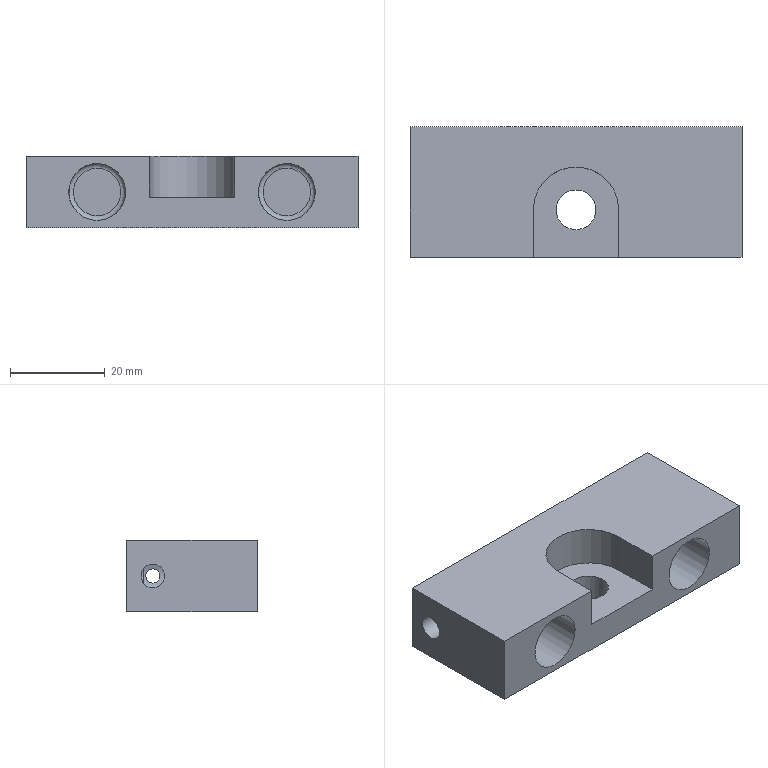NC program | NX | posted with a generic post | part box 70 x 27.5 x 15 mm
Lines 1624 to 2444 of 3352:
(PLANAR_MILL_2 , TOOL : D4-12-D4-50-3T-ROUGH)
N3228 T03 M6
N3230 G53
N3232 G17 G0 G90 X-5.038 Y-1.722 B0. C0. S3000 M3
N3234 G43 Z20. H3
N3236 Z-7.6
N3238 G94 G1 X-5.003 Y-1.751 Z-7.601 F600.
N3240 X-4.742 Y-1.911 Z-7.606
N3242 X-4.462 Y-2.032 Z-7.611
N3244 X-4.167 Y-2.112 Z-7.617
N3246 X-3.864 Y-2.15 Z-7.622
N3248 X-3.636 Z-7.626
N3250 X-3.333 Y-2.112 Z-7.631
N3252 X-3.038 Y-2.032 Z-7.637
N3254 X-2.758 Y-1.911 Z-7.642
N3256 X-2.497 Y-1.751 Z-7.647
N3258 X-2.262 Y-1.556 Z-7.653
N3260 X-2.057 Y-1.33 Z-7.658
N3262 X-1.885 Y-1.077 Z-7.663
N3264 X-1.752 Y-0.802 Z-7.669
N3266 X-1.658 Y-0.511 Z-7.674
N3268 X-1.607 Y-0.209 Z-7.679
N3270 X-1.599 Y0.096 Z-7.685
N3272 X-1.634 Y0.4 Z-7.69
N3274 X-1.712 Y0.695 Z-7.695
N3276 X-1.831 Y0.977 Z-7.701
N3278 X-1.945 Y1.173 Z-7.705
N3280 X-2.119 Y1.405 Z-7.71
N3282 X-2.322 Y1.611 Z-7.715
N3284 X-2.551 Y1.788 Z-7.72
N3286 X-2.801 Y1.933 Z-7.725
N3288 X-3.069 Y2.042 Z-7.73
N3290 X-3.349 Y2.115 Z-7.735
N3292 X-3.636 Y2.15 Z-7.74
N3294 X-3.864 Z-7.744
N3296 X-4.151 Y2.115 Z-7.749
N3298 X-4.431 Y2.042 Z-7.754
N3300 X-4.699 Y1.933 Z-7.759
N3302 X-4.949 Y1.788 Z-7.764
N3304 X-5.178 Y1.611 Z-7.769
N3306 X-5.381 Y1.405 Z-7.774
N3308 X-5.555 Y1.173 Z-7.779
N3310 X-5.669 Y0.977 Z-7.783
N3312 X-5.788 Y0.695 Z-7.789
N3314 X-5.866 Y0.4 Z-7.794
N3316 X-5.901 Y0.096 Z-7.799
N3318 X-5.893 Y-0.209 Z-7.805
N3320 X-5.842 Y-0.511 Z-7.81
N3322 X-5.748 Y-0.802 Z-7.815
N3324 X-5.615 Y-1.077 Z-7.821
N3326 X-5.443 Y-1.33 Z-7.826
N3328 X-5.238 Y-1.556 Z-7.831
N3330 X-5.003 Y-1.751 Z-7.837
N3332 X-4.742 Y-1.911 Z-7.842
N3334 X-4.462 Y-2.032 Z-7.847
N3336 X-4.167 Y-2.112 Z-7.853
N3338 X-3.864 Y-2.15 Z-7.858
N3340 X-3.636 Z-7.862
N3342 X-3.333 Y-2.112 Z-7.867
N3344 X-3.038 Y-2.032 Z-7.873
N3346 X-2.758 Y-1.911 Z-7.878
N3348 X-2.497 Y-1.751 Z-7.883
N3350 X-2.262 Y-1.556 Z-7.889
N3352 X-2.057 Y-1.33 Z-7.894
N3354 X-1.885 Y-1.077 Z-7.899
N3356 X-1.752 Y-0.802 Z-7.905
N3358 X-1.658 Y-0.511 Z-7.91
N3360 X-1.607 Y-0.209 Z-7.915
N3362 X-1.599 Y0.096 Z-7.921
N3364 X-1.634 Y0.4 Z-7.926
N3366 X-1.712 Y0.695 Z-7.931
N3368 X-1.831 Y0.977 Z-7.937
N3370 X-1.945 Y1.173 Z-7.941
N3372 X-2.119 Y1.405 Z-7.946
N3374 X-2.322 Y1.611 Z-7.951
N3376 X-2.551 Y1.788 Z-7.956
N3378 X-2.801 Y1.933 Z-7.961
N3380 X-3.069 Y2.042 Z-7.966
N3382 X-3.349 Y2.115 Z-7.971
N3384 X-3.636 Y2.15 Z-7.976
N3386 X-3.864 Z-7.98
N3388 X-4.151 Y2.115 Z-7.985
N3390 X-4.431 Y2.042 Z-7.99
N3392 X-4.699 Y1.933 Z-7.995
N3394 X-4.949 Y1.788 Z-8.
N3396 X-5.178 Y1.611 Z-8.005
N3398 X-5.381 Y1.405 Z-8.01
N3400 X-5.555 Y1.173 Z-8.015
N3402 X-5.669 Y0.977 Z-8.019
N3404 X-5.788 Y0.695 Z-8.025
N3406 X-5.866 Y0.4 Z-8.03
N3408 X-5.901 Y0.096 Z-8.035
N3410 X-5.893 Y-0.209 Z-8.041
N3412 X-5.842 Y-0.511 Z-8.046
N3414 X-5.748 Y-0.802 Z-8.051
N3416 X-5.615 Y-1.077 Z-8.057
N3418 X-5.443 Y-1.33 Z-8.062
N3420 X-5.238 Y-1.556 Z-8.067
N3422 X-5.003 Y-1.751 Z-8.073
N3424 X-4.742 Y-1.911 Z-8.078
N3426 X-4.462 Y-2.032 Z-8.083
N3428 X-4.167 Y-2.112 Z-8.089
N3430 X-3.864 Y-2.15 Z-8.094
N3432 X-3.636 Z-8.098
N3434 X-3.333 Y-2.112 Z-8.103
N3436 X-3.038 Y-2.032 Z-8.109
N3438 X-2.758 Y-1.911 Z-8.114
N3440 X-2.497 Y-1.751 Z-8.119
N3442 X-2.262 Y-1.556 Z-8.125
N3444 X-2.057 Y-1.33 Z-8.13
N3446 X-1.885 Y-1.077 Z-8.135
N3448 X-1.752 Y-0.802 Z-8.141
N3450 X-1.658 Y-0.511 Z-8.146
N3452 X-1.607 Y-0.209 Z-8.151
N3454 X-1.599 Y0.096 Z-8.157
N3456 X-1.634 Y0.4 Z-8.162
N3458 X-1.712 Y0.695 Z-8.167
N3460 X-1.831 Y0.977 Z-8.173
N3462 X-1.945 Y1.173 Z-8.177
N3464 X-2.119 Y1.405 Z-8.182
N3466 X-2.322 Y1.611 Z-8.187
N3468 X-2.551 Y1.788 Z-8.192
N3470 X-2.801 Y1.933 Z-8.197
N3472 X-3.069 Y2.042 Z-8.202
N3474 X-3.349 Y2.115 Z-8.207
N3476 X-3.636 Y2.15 Z-8.212
N3478 X-3.864 Z-8.216
N3480 X-4.151 Y2.115 Z-8.221
N3482 X-4.431 Y2.042 Z-8.226
N3484 X-4.699 Y1.933 Z-8.231
N3486 X-4.949 Y1.788 Z-8.236
N3488 X-5.178 Y1.611 Z-8.241
N3490 X-5.381 Y1.405 Z-8.246
N3492 X-5.555 Y1.173 Z-8.251
N3494 X-5.669 Y0.977 Z-8.255
N3496 X-5.788 Y0.695 Z-8.261
N3498 X-5.866 Y0.4 Z-8.266
N3500 X-5.901 Y0.096 Z-8.271
N3502 X-5.893 Y-0.209 Z-8.277
N3504 X-5.842 Y-0.511 Z-8.282
N3506 X-5.748 Y-0.802 Z-8.287
N3508 X-5.615 Y-1.077 Z-8.293
N3510 X-5.443 Y-1.33 Z-8.298
N3512 X-5.238 Y-1.556 Z-8.303
N3514 X-5.003 Y-1.751 Z-8.309
N3516 X-4.742 Y-1.911 Z-8.314
N3518 X-4.462 Y-2.032 Z-8.319
N3520 X-4.167 Y-2.112 Z-8.325
N3522 X-3.864 Y-2.15 Z-8.33
N3524 X-3.636 Z-8.334
N3526 X-3.333 Y-2.112 Z-8.339
N3528 X-3.038 Y-2.032 Z-8.345
N3530 X-2.758 Y-1.911 Z-8.35
N3532 X-2.497 Y-1.751 Z-8.355
N3534 X-2.262 Y-1.556 Z-8.361
N3536 X-2.057 Y-1.33 Z-8.366
N3538 X-1.885 Y-1.077 Z-8.371
N3540 X-1.752 Y-0.802 Z-8.377
N3542 X-1.658 Y-0.511 Z-8.382
N3544 X-1.607 Y-0.209 Z-8.387
N3546 X-1.599 Y0.096 Z-8.393
N3548 X-1.634 Y0.4 Z-8.398
N3550 X-1.712 Y0.695 Z-8.403
N3552 X-1.831 Y0.977 Z-8.409
N3554 X-1.945 Y1.173 Z-8.413
N3556 X-2.119 Y1.405 Z-8.418
N3558 X-2.322 Y1.611 Z-8.423
N3560 X-2.551 Y1.788 Z-8.428
N3562 X-2.801 Y1.933 Z-8.433
N3564 X-3.069 Y2.042 Z-8.438
N3566 X-3.349 Y2.115 Z-8.443
N3568 X-3.636 Y2.15 Z-8.448
N3570 X-3.864 Z-8.452
N3572 X-4.151 Y2.115 Z-8.457
N3574 X-4.431 Y2.042 Z-8.462
N3576 X-4.699 Y1.933 Z-8.467
N3578 X-4.949 Y1.788 Z-8.472
N3580 X-5.178 Y1.611 Z-8.477
N3582 X-5.381 Y1.405 Z-8.482
N3584 X-5.555 Y1.173 Z-8.487
N3586 X-5.669 Y0.977 Z-8.491
N3588 X-5.788 Y0.695 Z-8.497
N3590 X-5.866 Y0.4 Z-8.502
N3592 X-5.901 Y0.096 Z-8.507
N3594 X-5.893 Y-0.209 Z-8.513
N3596 X-5.842 Y-0.511 Z-8.518
N3598 X-5.748 Y-0.802 Z-8.523
N3600 X-5.615 Y-1.077 Z-8.529
N3602 X-5.443 Y-1.33 Z-8.534
N3604 X-5.238 Y-1.556 Z-8.539
N3606 X-5.003 Y-1.751 Z-8.545
N3608 X-4.742 Y-1.911 Z-8.55
N3610 X-4.462 Y-2.032 Z-8.555
N3612 X-4.167 Y-2.112 Z-8.561
N3614 X-3.864 Y-2.15 Z-8.566
N3616 X-3.636 Z-8.57
N3618 X-3.333 Y-2.112 Z-8.575
N3620 X-3.038 Y-2.032 Z-8.581
N3622 X-2.758 Y-1.911 Z-8.586
N3624 X-2.497 Y-1.751 Z-8.591
N3626 X-2.262 Y-1.556 Z-8.597
N3628 X-2.057 Y-1.33 Z-8.602
N3630 X-1.885 Y-1.077 Z-8.607
N3632 X-1.752 Y-0.802 Z-8.613
N3634 X-1.658 Y-0.511 Z-8.618
N3636 X-1.607 Y-0.209 Z-8.623
N3638 X-1.599 Y0.096 Z-8.629
N3640 X-1.634 Y0.4 Z-8.634
N3642 X-1.712 Y0.695 Z-8.639
N3644 X-1.831 Y0.977 Z-8.645
N3646 X-1.945 Y1.173 Z-8.649
N3648 X-2.119 Y1.405 Z-8.654
N3650 X-2.322 Y1.611 Z-8.659
N3652 X-2.551 Y1.788 Z-8.664
N3654 X-2.801 Y1.933 Z-8.669
N3656 X-3.069 Y2.042 Z-8.674
N3658 X-3.349 Y2.115 Z-8.679
N3660 X-3.636 Y2.15 Z-8.684
N3662 X-3.864 Z-8.688
N3664 X-4.151 Y2.115 Z-8.693
N3666 X-4.431 Y2.042 Z-8.698
N3668 X-4.699 Y1.933 Z-8.703
N3670 X-4.949 Y1.788 Z-8.708
N3672 X-5.178 Y1.611 Z-8.713
N3674 X-5.381 Y1.405 Z-8.718
N3676 X-5.555 Y1.173 Z-8.723
N3678 X-5.669 Y0.977 Z-8.727
N3680 X-5.788 Y0.695 Z-8.732
N3682 X-5.866 Y0.4 Z-8.738
N3684 X-5.901 Y0.096 Z-8.743
N3686 X-5.893 Y-0.209 Z-8.748
N3688 X-5.842 Y-0.511 Z-8.754
N3690 X-5.748 Y-0.802 Z-8.759
N3692 X-5.615 Y-1.077 Z-8.764
N3694 X-5.443 Y-1.33 Z-8.77
N3696 X-5.238 Y-1.556 Z-8.775
N3698 X-5.003 Y-1.751 Z-8.78
N3700 X-4.742 Y-1.911 Z-8.786
N3702 X-4.462 Y-2.032 Z-8.791
N3704 X-4.167 Y-2.112 Z-8.796
N3706 X-3.864 Y-2.15 Z-8.802
N3708 X-3.636 Z-8.806
N3710 X-3.333 Y-2.112 Z-8.811
N3712 X-3.038 Y-2.032 Z-8.816
N3714 X-2.758 Y-1.911 Z-8.822
N3716 X-2.497 Y-1.751 Z-8.827
N3718 X-2.262 Y-1.556 Z-8.832
N3720 X-2.057 Y-1.33 Z-8.838
N3722 X-1.885 Y-1.077 Z-8.843
N3724 X-1.752 Y-0.802 Z-8.848
N3726 X-1.658 Y-0.511 Z-8.854
N3728 X-1.607 Y-0.209 Z-8.859
N3730 X-1.599 Y0.096 Z-8.864
N3732 X-1.634 Y0.4 Z-8.87
N3734 X-1.712 Y0.695 Z-8.875
N3736 X-1.831 Y0.977 Z-8.88
N3738 X-1.945 Y1.173 Z-8.884
N3740 X-2.119 Y1.405 Z-8.889
N3742 X-2.322 Y1.611 Z-8.895
N3744 X-2.551 Y1.788 Z-8.9
N3746 X-2.801 Y1.933 Z-8.905
N3748 X-3.069 Y2.042 Z-8.91
N3750 X-3.349 Y2.115 Z-8.915
N3752 X-3.636 Y2.15 Z-8.92
N3754 X-3.864 Z-8.924
N3756 X-4.151 Y2.115 Z-8.929
N3758 X-4.431 Y2.042 Z-8.934
N3760 X-4.699 Y1.933 Z-8.939
N3762 X-4.949 Y1.788 Z-8.944
N3764 X-5.178 Y1.611 Z-8.949
N3766 X-5.381 Y1.405 Z-8.954
N3768 X-5.555 Y1.173 Z-8.959
N3770 X-5.669 Y0.977 Z-8.963
N3772 X-5.788 Y0.695 Z-8.968
N3774 X-5.866 Y0.4 Z-8.974
N3776 X-5.901 Y0.096 Z-8.979
N3778 X-5.893 Y-0.209 Z-8.984
N3780 X-5.842 Y-0.511 Z-8.99
N3782 X-5.748 Y-0.802 Z-8.995
N3784 X-5.615 Y-1.077 Z-9.
N3786 X-5.443 Y-1.33 Z-9.006
N3788 X-5.238 Y-1.556 Z-9.011
N3790 X-5.003 Y-1.751 Z-9.016
N3792 X-4.742 Y-1.911 Z-9.022
N3794 X-4.462 Y-2.032 Z-9.027
N3796 X-4.167 Y-2.112 Z-9.032
N3798 X-3.864 Y-2.15 Z-9.038
N3800 X-3.636 Z-9.042
N3802 X-3.333 Y-2.112 Z-9.047
N3804 X-3.038 Y-2.032 Z-9.052
N3806 X-2.758 Y-1.911 Z-9.058
N3808 X-2.497 Y-1.751 Z-9.063
N3810 X-2.262 Y-1.556 Z-9.068
N3812 X-2.057 Y-1.33 Z-9.074
N3814 X-1.885 Y-1.077 Z-9.079
N3816 X-1.752 Y-0.802 Z-9.084
N3818 X-1.658 Y-0.511 Z-9.09
N3820 X-1.607 Y-0.209 Z-9.095
N3822 X-1.599 Y0.096 Z-9.1
N3824 X-1.634 Y0.4 Z-9.106
N3826 X-1.712 Y0.695 Z-9.111
N3828 X-1.831 Y0.977 Z-9.116
N3830 X-1.945 Y1.173 Z-9.12
N3832 X-2.119 Y1.405 Z-9.125
N3834 X-2.322 Y1.611 Z-9.13
N3836 X-2.551 Y1.788 Z-9.136
N3838 X-2.801 Y1.933 Z-9.141
N3840 X-3.069 Y2.042 Z-9.146
N3842 X-3.349 Y2.115 Z-9.151
N3844 X-3.636 Y2.15 Z-9.156
N3846 X-3.864 Z-9.16
N3848 X-4.151 Y2.115 Z-9.165
N3850 X-4.431 Y2.042 Z-9.17
N3852 X-4.699 Y1.933 Z-9.175
N3854 X-4.949 Y1.788 Z-9.18
N3856 X-5.178 Y1.611 Z-9.185
N3858 X-5.381 Y1.405 Z-9.19
N3860 X-5.555 Y1.173 Z-9.195
N3862 X-5.669 Y0.977 Z-9.199
N3864 X-5.788 Y0.695 Z-9.204
N3866 X-5.866 Y0.4 Z-9.21
N3868 X-5.901 Y0.096 Z-9.215
N3870 X-5.893 Y-0.209 Z-9.22
N3872 X-5.842 Y-0.511 Z-9.226
N3874 X-5.748 Y-0.802 Z-9.231
N3876 X-5.615 Y-1.077 Z-9.236
N3878 X-5.443 Y-1.33 Z-9.242
N3880 X-5.238 Y-1.556 Z-9.247
N3882 X-5.003 Y-1.751 Z-9.252
N3884 X-4.742 Y-1.911 Z-9.258
N3886 X-4.462 Y-2.032 Z-9.263
N3888 X-4.167 Y-2.112 Z-9.268
N3890 X-3.864 Y-2.15 Z-9.274
N3892 X-3.636 Z-9.278
N3894 X-3.333 Y-2.112 Z-9.283
N3896 X-3.038 Y-2.032 Z-9.288
N3898 X-2.758 Y-1.911 Z-9.294
N3900 X-2.497 Y-1.751 Z-9.299
N3902 X-2.262 Y-1.556 Z-9.304
N3904 X-2.057 Y-1.33 Z-9.31
N3906 X-1.885 Y-1.077 Z-9.315
N3908 X-1.752 Y-0.802 Z-9.32
N3910 X-1.658 Y-0.511 Z-9.326
N3912 X-1.607 Y-0.209 Z-9.331
N3914 X-1.599 Y0.096 Z-9.336
N3916 X-1.634 Y0.4 Z-9.342
N3918 X-1.712 Y0.695 Z-9.347
N3920 X-1.831 Y0.977 Z-9.352
N3922 X-1.945 Y1.173 Z-9.356
N3924 X-2.119 Y1.405 Z-9.361
N3926 X-2.322 Y1.611 Z-9.366
N3928 X-2.551 Y1.788 Z-9.371
N3930 X-2.801 Y1.933 Z-9.377
N3932 X-3.069 Y2.042 Z-9.382
N3934 X-3.349 Y2.115 Z-9.387
N3936 X-3.636 Y2.15 Z-9.392
N3938 X-3.864 Z-9.396
N3940 X-4.151 Y2.115 Z-9.401
N3942 X-4.431 Y2.042 Z-9.406
N3944 X-4.699 Y1.933 Z-9.411
N3946 X-4.949 Y1.788 Z-9.416
N3948 X-5.178 Y1.611 Z-9.421
N3950 X-5.381 Y1.405 Z-9.426
N3952 X-5.555 Y1.173 Z-9.431
N3954 X-5.669 Y0.977 Z-9.435
N3956 X-5.788 Y0.695 Z-9.44
N3958 X-5.866 Y0.4 Z-9.446
N3960 X-5.901 Y0.096 Z-9.451
N3962 X-5.893 Y-0.209 Z-9.456
N3964 X-5.842 Y-0.511 Z-9.462
N3966 X-5.748 Y-0.802 Z-9.467
N3968 X-5.615 Y-1.077 Z-9.472
N3970 X-5.443 Y-1.33 Z-9.478
N3972 X-5.238 Y-1.556 Z-9.483
N3974 X-5.003 Y-1.751 Z-9.488
N3976 X-4.742 Y-1.911 Z-9.494
N3978 X-4.462 Y-2.032 Z-9.499
N3980 X-4.167 Y-2.112 Z-9.504
N3982 X-3.864 Y-2.15 Z-9.51
N3984 X-3.636 Z-9.514
N3986 X-3.333 Y-2.112 Z-9.519
N3988 X-3.038 Y-2.032 Z-9.524
N3990 X-2.758 Y-1.911 Z-9.53
N3992 X-2.497 Y-1.751 Z-9.535
N3994 X-2.262 Y-1.556 Z-9.54
N3996 X-2.057 Y-1.33 Z-9.546
N3998 X-1.885 Y-1.077 Z-9.551
N4000 X-1.752 Y-0.802 Z-9.556
N4002 X-1.658 Y-0.511 Z-9.562
N4004 X-1.607 Y-0.209 Z-9.567
N4006 X-1.599 Y0.096 Z-9.572
N4008 X-1.634 Y0.4 Z-9.578
N4010 X-1.712 Y0.695 Z-9.583
N4012 X-1.831 Y0.977 Z-9.588
N4014 X-1.945 Y1.173 Z-9.592
N4016 X-2.119 Y1.405 Z-9.597
N4018 X-2.322 Y1.611 Z-9.602
N4020 X-2.551 Y1.788 Z-9.607
N4022 X-2.801 Y1.933 Z-9.612
N4024 X-3.069 Y2.042 Z-9.618
N4026 X-3.349 Y2.115 Z-9.623
N4028 X-3.636 Y2.15 Z-9.628
N4030 X-3.864 Z-9.632
N4032 X-4.151 Y2.115 Z-9.637
N4034 X-4.431 Y2.042 Z-9.642
N4036 X-4.699 Y1.933 Z-9.647
N4038 X-4.949 Y1.788 Z-9.652
N4040 X-5.178 Y1.611 Z-9.657
N4042 X-5.381 Y1.405 Z-9.662
N4044 X-5.555 Y1.173 Z-9.667
N4046 X-5.669 Y0.977 Z-9.671
N4048 X-5.788 Y0.695 Z-9.676
N4050 X-5.866 Y0.4 Z-9.682
N4052 X-5.901 Y0.096 Z-9.687
N4054 X-5.893 Y-0.209 Z-9.692
N4056 X-5.842 Y-0.511 Z-9.698
N4058 X-5.748 Y-0.802 Z-9.703
N4060 X-5.615 Y-1.077 Z-9.708
N4062 X-5.443 Y-1.33 Z-9.714
N4064 X-5.238 Y-1.556 Z-9.719
N4066 X-5.003 Y-1.751 Z-9.724
N4068 X-4.742 Y-1.911 Z-9.73
N4070 X-4.462 Y-2.032 Z-9.735
N4072 X-4.167 Y-2.112 Z-9.74
N4074 X-3.864 Y-2.15 Z-9.746
N4076 X-3.636 Z-9.75
N4078 X-3.333 Y-2.112 Z-9.755
N4080 X-3.038 Y-2.032 Z-9.76
N4082 X-2.758 Y-1.911 Z-9.766
N4084 X-2.497 Y-1.751 Z-9.771
N4086 X-2.262 Y-1.556 Z-9.776
N4088 X-2.057 Y-1.33 Z-9.782
N4090 X-1.885 Y-1.077 Z-9.787
N4092 X-1.752 Y-0.802 Z-9.792
N4094 X-1.658 Y-0.511 Z-9.798
N4096 X-1.607 Y-0.209 Z-9.803
N4098 X-1.599 Y0.096 Z-9.808
N4100 X-1.634 Y0.4 Z-9.814
N4102 X-1.712 Y0.695 Z-9.819
N4104 X-1.831 Y0.977 Z-9.824
N4106 X-1.945 Y1.173 Z-9.828
N4108 X-2.119 Y1.405 Z-9.833
N4110 X-2.322 Y1.611 Z-9.838
N4112 X-2.551 Y1.788 Z-9.843
N4114 X-2.801 Y1.933 Z-9.848
N4116 X-3.069 Y2.042 Z-9.853
N4118 X-3.349 Y2.115 Z-9.859
N4120 X-3.636 Y2.15 Z-9.864
N4122 X-3.864 Z-9.868
N4124 X-4.151 Y2.115 Z-9.873
N4126 X-4.431 Y2.042 Z-9.878
N4128 X-4.699 Y1.933 Z-9.883
N4130 X-4.949 Y1.788 Z-9.888
N4132 X-5.178 Y1.611 Z-9.893
N4134 X-5.381 Y1.405 Z-9.898
N4136 X-5.555 Y1.173 Z-9.903
N4138 X-5.669 Y0.977 Z-9.907
N4140 X-5.788 Y0.695 Z-9.912
N4142 X-5.866 Y0.4 Z-9.918
N4144 X-5.901 Y0.096 Z-9.923
N4146 X-5.893 Y-0.209 Z-9.928
N4148 X-5.842 Y-0.511 Z-9.934
N4150 X-5.748 Y-0.802 Z-9.939
N4152 X-5.615 Y-1.077 Z-9.944
N4154 X-5.443 Y-1.33 Z-9.95
N4156 X-5.238 Y-1.556 Z-9.955
N4158 X-5.003 Y-1.751 Z-9.96
N4160 X-4.742 Y-1.911 Z-9.966
N4162 X-4.462 Y-2.032 Z-9.971
N4164 X-4.167 Y-2.112 Z-9.976
N4166 X-3.864 Y-2.15 Z-9.982
N4168 X-3.636 Z-9.986
N4170 X-3.333 Y-2.112 Z-9.991
N4172 X-3.038 Y-2.032 Z-9.996
N4174 X-2.758 Y-1.911 Z-10.002
N4176 X-2.497 Y-1.751 Z-10.007
N4178 X-2.262 Y-1.556 Z-10.012
N4180 X-2.057 Y-1.33 Z-10.018
N4182 X-1.885 Y-1.077 Z-10.023
N4184 X-1.752 Y-0.802 Z-10.028
N4186 X-1.658 Y-0.511 Z-10.034
N4188 X-1.607 Y-0.209 Z-10.039
N4190 X-1.599 Y0.096 Z-10.044
N4192 X-1.634 Y0.4 Z-10.05
N4194 X-1.712 Y0.695 Z-10.055
N4196 X-1.831 Y0.977 Z-10.06
N4198 X-1.945 Y1.173 Z-10.064
N4200 X-2.119 Y1.405 Z-10.069
N4202 X-2.322 Y1.611 Z-10.074
N4204 X-2.551 Y1.788 Z-10.079
N4206 X-2.801 Y1.933 Z-10.084
N4208 X-3.069 Y2.042 Z-10.089
N4210 X-3.349 Y2.115 Z-10.094
N4212 X-3.636 Y2.15 Z-10.1
N4214 X-3.864 Z-10.103
N4216 X-4.151 Y2.115 Z-10.109
N4218 X-4.431 Y2.042 Z-10.114
N4220 X-4.699 Y1.933 Z-10.119
N4222 X-4.949 Y1.788 Z-10.124
N4224 X-5.178 Y1.611 Z-10.129
N4226 X-5.381 Y1.405 Z-10.134
N4228 X-5.555 Y1.173 Z-10.139
N4230 X-5.669 Y0.977 Z-10.143
N4232 X-5.788 Y0.695 Z-10.148
N4234 X-5.866 Y0.4 Z-10.153
N4236 X-5.901 Y0.096 Z-10.159
N4238 X-5.893 Y-0.209 Z-10.164
N4240 X-5.842 Y-0.511 Z-10.169
N4242 X-5.748 Y-0.802 Z-10.175
N4244 X-5.615 Y-1.077 Z-10.18
N4246 X-5.443 Y-1.33 Z-10.185
N4248 X-5.238 Y-1.556 Z-10.191
N4250 X-5.003 Y-1.751 Z-10.196
N4252 X-4.742 Y-1.911 Z-10.201
N4254 X-4.462 Y-2.032 Z-10.207
N4256 X-4.167 Y-2.112 Z-10.212
N4258 X-3.864 Y-2.15 Z-10.217
N4260 X-3.636 Z-10.221
N4262 X-3.333 Y-2.112 Z-10.227
N4264 X-3.038 Y-2.032 Z-10.232
N4266 X-2.758 Y-1.911 Z-10.237
N4268 X-2.497 Y-1.751 Z-10.243
N4270 X-2.262 Y-1.556 Z-10.248
N4272 X-2.057 Y-1.33 Z-10.253
N4274 X-1.885 Y-1.077 Z-10.259
N4276 X-1.752 Y-0.802 Z-10.264
N4278 X-1.658 Y-0.511 Z-10.269
N4280 X-1.607 Y-0.209 Z-10.275
N4282 X-1.599 Y0.096 Z-10.28
N4284 X-1.634 Y0.4 Z-10.285
N4286 X-1.712 Y0.695 Z-10.291
N4288 X-1.831 Y0.977 Z-10.296
N4290 X-1.945 Y1.173 Z-10.3
N4292 X-2.119 Y1.405 Z-10.305
N4294 X-2.322 Y1.611 Z-10.31
N4296 X-2.551 Y1.788 Z-10.315
N4298 X-2.801 Y1.933 Z-10.32
N4300 X-3.069 Y2.042 Z-10.325
N4302 X-3.349 Y2.115 Z-10.33
N4304 X-3.636 Y2.15 Z-10.335
N4306 X-3.864 Z-10.339
N4308 X-4.151 Y2.115 Z-10.344
N4310 X-4.431 Y2.042 Z-10.35
N4312 X-4.699 Y1.933 Z-10.355
N4314 X-4.949 Y1.788 Z-10.36
N4316 X-5.178 Y1.611 Z-10.365
N4318 X-5.381 Y1.405 Z-10.37
N4320 X-5.555 Y1.173 Z-10.375
N4322 X-5.669 Y0.977 Z-10.379
N4324 X-5.788 Y0.695 Z-10.384
N4326 X-5.866 Y0.4 Z-10.389
N4328 X-5.901 Y0.096 Z-10.395
N4330 X-5.893 Y-0.209 Z-10.4
N4332 X-5.842 Y-0.511 Z-10.405
N4334 X-5.748 Y-0.802 Z-10.411
N4336 X-5.615 Y-1.077 Z-10.416
N4338 X-5.443 Y-1.33 Z-10.421
N4340 X-5.238 Y-1.556 Z-10.427
N4342 X-5.003 Y-1.751 Z-10.432
N4344 X-4.742 Y-1.911 Z-10.437
N4346 X-4.462 Y-2.032 Z-10.443
N4348 X-4.167 Y-2.112 Z-10.448
N4350 X-3.864 Y-2.15 Z-10.453
N4352 X-3.636 Z-10.457
N4354 X-3.333 Y-2.112 Z-10.463
N4356 X-3.038 Y-2.032 Z-10.468
N4358 X-2.758 Y-1.911 Z-10.473
N4360 X-2.497 Y-1.751 Z-10.479
N4362 X-2.262 Y-1.556 Z-10.484
N4364 X-2.057 Y-1.33 Z-10.489
N4366 X-1.885 Y-1.077 Z-10.495
N4368 X-1.752 Y-0.802 Z-10.5
N4370 X-1.658 Y-0.511 Z-10.505
N4372 X-1.607 Y-0.209 Z-10.511
N4374 X-1.599 Y0.096 Z-10.516
N4376 X-1.634 Y0.4 Z-10.521
N4378 X-1.712 Y0.695 Z-10.527
N4380 X-1.831 Y0.977 Z-10.532
N4382 X-1.945 Y1.173 Z-10.536
N4384 X-2.119 Y1.405 Z-10.541
N4386 X-2.322 Y1.611 Z-10.546
N4388 X-2.551 Y1.788 Z-10.551
N4390 X-2.801 Y1.933 Z-10.556
N4392 X-3.069 Y2.042 Z-10.561
N4394 X-3.349 Y2.115 Z-10.566
N4396 X-3.636 Y2.15 Z-10.571
N4398 X-3.864 Z-10.575
N4400 X-4.151 Y2.115 Z-10.58
N4402 X-4.431 Y2.042 Z-10.585
N4404 X-4.699 Y1.933 Z-10.591
N4406 X-4.949 Y1.788 Z-10.596
N4408 X-5.178 Y1.611 Z-10.601
N4410 X-5.381 Y1.405 Z-10.606
N4412 X-5.555 Y1.173 Z-10.611
N4414 X-5.669 Y0.977 Z-10.615
N4416 X-5.788 Y0.695 Z-10.62
N4418 X-5.866 Y0.4 Z-10.625
N4420 X-5.901 Y0.096 Z-10.631
N4422 X-5.893 Y-0.209 Z-10.636
N4424 X-5.842 Y-0.511 Z-10.641
N4426 X-5.748 Y-0.802 Z-10.647
N4428 X-5.615 Y-1.077 Z-10.652
N4430 X-5.443 Y-1.33 Z-10.657
N4432 X-5.238 Y-1.556 Z-10.663
N4434 X-5.003 Y-1.751 Z-10.668
N4436 X-4.742 Y-1.911 Z-10.673
N4438 X-4.462 Y-2.032 Z-10.679
N4440 X-4.167 Y-2.112 Z-10.684
N4442 X-3.864 Y-2.15 Z-10.689
N4444 X-3.636 Z-10.693
N4446 X-3.333 Y-2.112 Z-10.699
N4448 X-3.038 Y-2.032 Z-10.704
N4450 X-2.758 Y-1.911 Z-10.709
N4452 X-2.497 Y-1.751 Z-10.715
N4454 X-2.262 Y-1.556 Z-10.72
N4456 X-2.057 Y-1.33 Z-10.725
N4458 X-1.885 Y-1.077 Z-10.731
N4460 X-1.752 Y-0.802 Z-10.736
N4462 X-1.658 Y-0.511 Z-10.741
N4464 X-1.607 Y-0.209 Z-10.747
N4466 X-1.599 Y0.096 Z-10.752
N4468 X-1.634 Y0.4 Z-10.757
N4470 X-1.712 Y0.695 Z-10.763
N4472 X-1.831 Y0.977 Z-10.768
N4474 X-1.945 Y1.173 Z-10.772
N4476 X-2.119 Y1.405 Z-10.777
N4478 X-2.322 Y1.611 Z-10.782
N4480 X-2.551 Y1.788 Z-10.787
N4482 X-2.801 Y1.933 Z-10.792
N4484 X-3.069 Y2.042 Z-10.797
N4486 X-3.349 Y2.115 Z-10.802
N4488 X-3.636 Y2.15 Z-10.807
N4490 X-3.864 Z-10.811
N4492 X-4.151 Y2.115 Z-10.816
N4494 X-4.431 Y2.042 Z-10.821
N4496 X-4.699 Y1.933 Z-10.826
N4498 X-4.949 Y1.788 Z-10.831
N4500 X-5.178 Y1.611 Z-10.837
N4502 X-5.381 Y1.405 Z-10.842
N4504 X-5.555 Y1.173 Z-10.847
N4506 X-5.669 Y0.977 Z-10.851
N4508 X-5.788 Y0.695 Z-10.856
N4510 X-5.866 Y0.4 Z-10.861
N4512 X-5.901 Y0.096 Z-10.867
N4514 X-5.893 Y-0.209 Z-10.872
N4516 X-5.842 Y-0.511 Z-10.877
N4518 X-5.748 Y-0.802 Z-10.883
N4520 X-5.615 Y-1.077 Z-10.888
N4522 X-5.443 Y-1.33 Z-10.893
N4524 X-5.238 Y-1.556 Z-10.899
N4526 X-5.003 Y-1.751 Z-10.904
N4528 X-4.742 Y-1.911 Z-10.909
N4530 X-4.462 Y-2.032 Z-10.915
N4532 X-4.167 Y-2.112 Z-10.92
N4534 X-3.864 Y-2.15 Z-10.925
N4536 X-3.636 Z-10.929
N4538 X-3.333 Y-2.112 Z-10.935
N4540 X-3.038 Y-2.032 Z-10.94
N4542 X-2.758 Y-1.911 Z-10.945
N4544 X-2.497 Y-1.751 Z-10.951
N4546 X-2.262 Y-1.556 Z-10.956
N4548 X-2.057 Y-1.33 Z-10.961
N4550 X-1.885 Y-1.077 Z-10.967
N4552 X-1.752 Y-0.802 Z-10.972
N4554 X-1.658 Y-0.511 Z-10.977
N4556 X-1.607 Y-0.209 Z-10.983
N4558 X-1.599 Y0.096 Z-10.988
N4560 X-1.634 Y0.4 Z-10.993
N4562 X-1.712 Y0.695 Z-10.999
N4564 X-1.831 Y0.977 Z-11.004
N4566 X-1.945 Y1.173 Z-11.008
N4568 X-2.119 Y1.405 Z-11.013
N4570 X-2.322 Y1.611 Z-11.018
N4572 X-2.551 Y1.788 Z-11.023
N4574 X-2.801 Y1.933 Z-11.028
N4576 X-3.069 Y2.042 Z-11.033
N4578 X-3.349 Y2.115 Z-11.038
N4580 X-3.636 Y2.15 Z-11.043
N4582 X-3.864 Z-11.047
N4584 X-4.151 Y2.115 Z-11.052
N4586 X-4.431 Y2.042 Z-11.057
N4588 X-4.699 Y1.933 Z-11.062
N4590 X-4.949 Y1.788 Z-11.067
N4592 X-5.178 Y1.611 Z-11.072
N4594 X-5.381 Y1.405 Z-11.078
N4596 X-5.555 Y1.173 Z-11.083
N4598 X-5.669 Y0.977 Z-11.087
N4600 X-5.788 Y0.695 Z-11.092
N4602 X-5.866 Y0.4 Z-11.097
N4604 X-5.901 Y0.096 Z-11.103
N4606 X-5.893 Y-0.209 Z-11.108
N4608 X-5.842 Y-0.511 Z-11.113
N4610 X-5.748 Y-0.802 Z-11.119
N4612 X-5.615 Y-1.077 Z-11.124
N4614 X-5.443 Y-1.33 Z-11.129
N4616 X-5.238 Y-1.556 Z-11.135
N4618 X-5.003 Y-1.751 Z-11.14
N4620 X-4.742 Y-1.911 Z-11.145
N4622 X-4.462 Y-2.032 Z-11.151
N4624 X-4.167 Y-2.112 Z-11.156
N4626 X-3.864 Y-2.15 Z-11.161
N4628 X-3.636 Z-11.165
N4630 X-3.333 Y-2.112 Z-11.171
N4632 X-3.038 Y-2.032 Z-11.176
N4634 X-2.758 Y-1.911 Z-11.181
N4636 X-2.497 Y-1.751 Z-11.187
N4638 X-2.262 Y-1.556 Z-11.192
N4640 X-2.057 Y-1.33 Z-11.197
N4642 X-1.885 Y-1.077 Z-11.203
N4644 X-1.752 Y-0.802 Z-11.208
N4646 X-1.658 Y-0.511 Z-11.213
N4648 X-1.607 Y-0.209 Z-11.219
N4650 X-1.599 Y0.096 Z-11.224
N4652 X-1.634 Y0.4 Z-11.229
N4654 X-1.712 Y0.695 Z-11.235
N4656 X-1.831 Y0.977 Z-11.24
N4658 X-1.945 Y1.173 Z-11.244
N4660 X-2.119 Y1.405 Z-11.249
N4662 X-2.322 Y1.611 Z-11.254
N4664 X-2.551 Y1.788 Z-11.259
N4666 X-2.801 Y1.933 Z-11.264
N4668 X-3.069 Y2.042 Z-11.269
N4670 X-3.349 Y2.115 Z-11.274
N4672 X-3.636 Y2.15 Z-11.279
N4674 X-3.864 Z-11.283
N4676 X-4.151 Y2.115 Z-11.288
N4678 X-4.431 Y2.042 Z-11.293
N4680 X-4.699 Y1.933 Z-11.298
N4682 X-4.949 Y1.788 Z-11.303
N4684 X-5.178 Y1.611 Z-11.308
N4686 X-5.381 Y1.405 Z-11.313
N4688 X-5.555 Y1.173 Z-11.319
N4690 X-5.669 Y0.977 Z-11.323
N4692 X-5.788 Y0.695 Z-11.328
N4694 X-5.866 Y0.4 Z-11.333
N4696 X-5.901 Y0.096 Z-11.339
N4698 X-5.893 Y-0.209 Z-11.344
N4700 X-5.842 Y-0.511 Z-11.349
N4702 X-5.748 Y-0.802 Z-11.355
N4704 X-5.615 Y-1.077 Z-11.36
N4706 X-5.443 Y-1.33 Z-11.365
N4708 X-5.238 Y-1.556 Z-11.371
N4710 X-5.003 Y-1.751 Z-11.376
N4712 X-4.742 Y-1.911 Z-11.381
N4714 X-4.462 Y-2.032 Z-11.387
N4716 X-4.167 Y-2.112 Z-11.392
N4718 X-3.864 Y-2.15 Z-11.397
N4720 X-3.636 Z-11.401
N4722 X-3.333 Y-2.112 Z-11.406
N4724 X-3.038 Y-2.032 Z-11.412
N4726 X-2.758 Y-1.911 Z-11.417
N4728 X-2.497 Y-1.751 Z-11.422
N4730 X-2.262 Y-1.556 Z-11.428
N4732 X-2.057 Y-1.33 Z-11.433
N4734 X-1.885 Y-1.077 Z-11.438
N4736 X-1.752 Y-0.802 Z-11.444
N4738 X-1.658 Y-0.511 Z-11.449
N4740 X-1.607 Y-0.209 Z-11.454
N4742 X-1.599 Y0.096 Z-11.46
N4744 X-1.634 Y0.4 Z-11.465
N4746 X-1.712 Y0.695 Z-11.47
N4748 X-1.831 Y0.977 Z-11.476
N4750 X-1.945 Y1.173 Z-11.48
N4752 X-2.119 Y1.405 Z-11.485
N4754 X-2.322 Y1.611 Z-11.49
N4756 X-2.551 Y1.788 Z-11.495
N4758 X-2.801 Y1.933 Z-11.5
N4760 X-3.069 Y2.042 Z-11.505
N4762 X-3.349 Y2.115 Z-11.51
N4764 X-3.636 Y2.15 Z-11.515
N4766 X-3.864 Z-11.519
N4768 X-4.151 Y2.115 Z-11.524
N4770 X-4.431 Y2.042 Z-11.529
N4772 X-4.699 Y1.933 Z-11.534
N4774 X-4.949 Y1.788 Z-11.539
N4776 X-5.178 Y1.611 Z-11.544
N4778 X-5.381 Y1.405 Z-11.549
N4780 X-5.555 Y1.173 Z-11.554
N4782 X-5.669 Y0.977 Z-11.558
N4784 X-5.788 Y0.695 Z-11.564
N4786 X-5.866 Y0.4 Z-11.569
N4788 X-5.901 Y0.096 Z-11.574
N4790 X-5.893 Y-0.209 Z-11.58
N4792 X-5.842 Y-0.511 Z-11.585
N4794 X-5.748 Y-0.802 Z-11.59
N4796 X-5.615 Y-1.077 Z-11.596
N4798 X-5.443 Y-1.33 Z-11.601
N4800 X-5.238 Y-1.556 Z-11.606
N4802 X-5.003 Y-1.751 Z-11.612
N4804 X-4.742 Y-1.911 Z-11.617
N4806 X-4.462 Y-2.032 Z-11.622
N4808 X-4.167 Y-2.112 Z-11.628
N4810 X-3.864 Y-2.15 Z-11.633
N4812 X-3.636 Z-11.637
N4814 X-3.333 Y-2.112 Z-11.642
N4816 X-3.038 Y-2.032 Z-11.648
N4818 X-2.758 Y-1.911 Z-11.653
N4820 X-2.497 Y-1.751 Z-11.658
N4822 X-2.262 Y-1.556 Z-11.664
N4824 X-2.057 Y-1.33 Z-11.669
N4826 X-1.885 Y-1.077 Z-11.674
N4828 X-1.752 Y-0.802 Z-11.68
N4830 X-1.658 Y-0.511 Z-11.685
N4832 X-1.607 Y-0.209 Z-11.69
N4834 X-1.599 Y0.096 Z-11.696
N4836 X-1.634 Y0.4 Z-11.701
N4838 X-1.712 Y0.695 Z-11.706
N4840 X-1.831 Y0.977 Z-11.712
N4842 X-1.945 Y1.173 Z-11.716
N4844 X-2.119 Y1.405 Z-11.721
N4846 X-2.322 Y1.611 Z-11.726
N4848 X-2.551 Y1.788 Z-11.731
N4850 X-2.801 Y1.933 Z-11.736
N4852 X-3.069 Y2.042 Z-11.741
N4854 X-3.349 Y2.115 Z-11.746
N4856 X-3.636 Y2.15 Z-11.751
N4858 X-3.864 Z-11.755
N4860 X-4.151 Y2.115 Z-11.76
N4862 X-4.431 Y2.042 Z-11.765